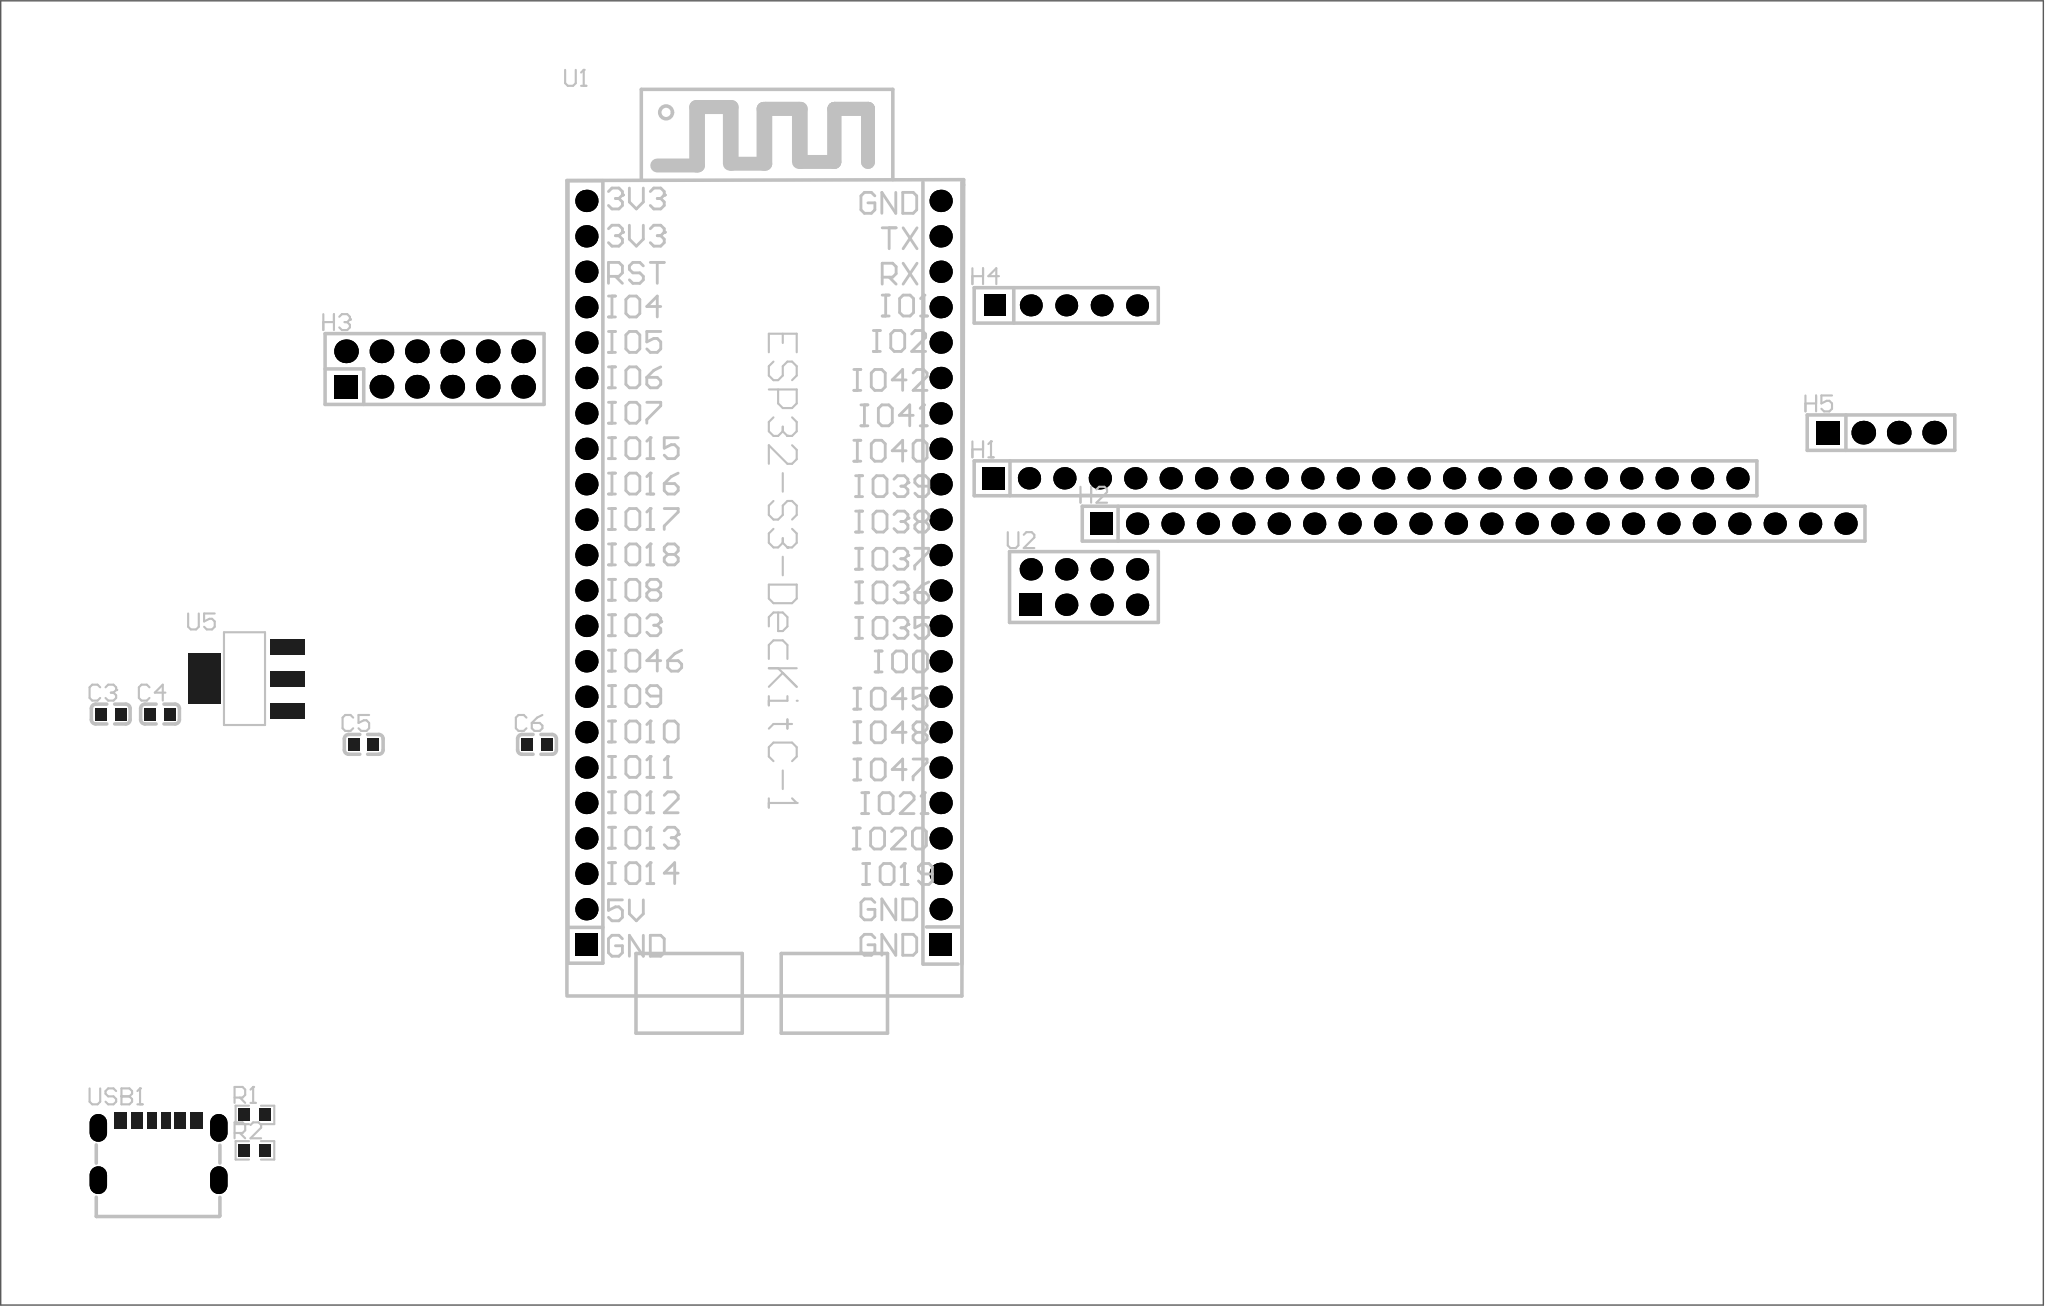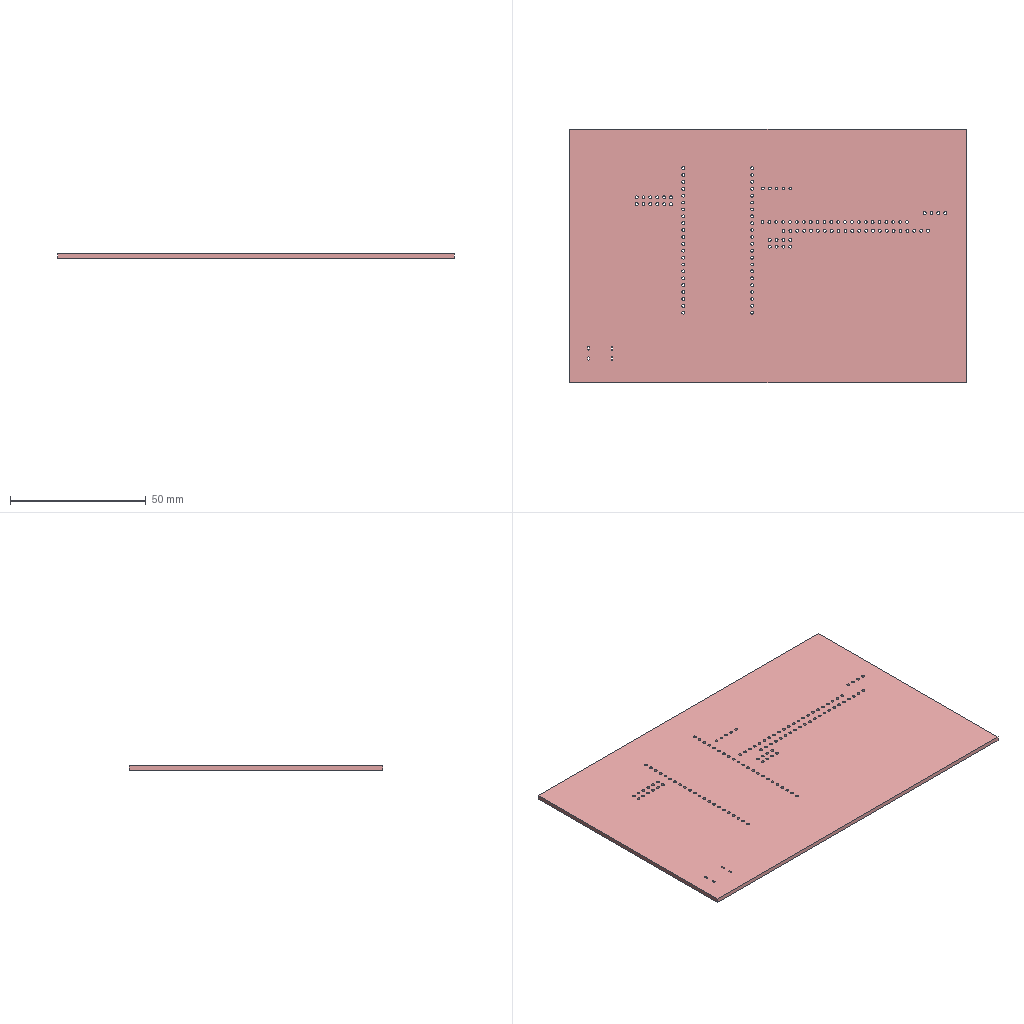Circuit board layout | Altium Designer | box 146.5 x 93.5 x 1.6 mm
Layer stack:
# Altium Designer layer stack of  (unit mm; dielectric type: 0 none, 1 core, 2 prepreg, 3 surface material)
index,name,kind,layer,copper_thickness_mm,dielectric_type,dielectric_thickness_mm,dielectric_material,dielectric_constant
0,Top Paste Mask Layer,other,,,,,,
1,Top Silkscreen Layer,other,,,,,,
2,Top Solder Mask Layer,dielectric,,,3,0.01,,3.3
3,Top Layer,copper,Top Layer,0.035,,,,
4,Dielectric1,dielectric,,,3,1.51,FR4,4.5
5,Bottom Layer,copper,Bottom Layer,0.035,,,,
6,Bottom Solder Mask Layer,dielectric,,,3,0.01,,3.3
7,Bottom Silkscreen Layer,other,,,,,,
8,Bottom Paste Mask Layer,other,,,,,,
# drill layer pairs: low layer,high layer
drill_pair,Top Layer,Bottom Layer
Part placement:
Designator,Comment,Layer,Footprint,Center-X(mm),Center-Y(mm),Rotation
C3,10uF,TopLayer,C0603,77.739,112.237,0
C4,100nF,TopLayer,C0603,81.273,112.237,0
C5,10uF,TopLayer,C0603,95.879,110.063,0
C6,100nF,TopLayer,C0603,108.303,110.063,0
H1,CS-1165SDIG-1*22,TopLayer,HDR-TH_22P-P2.54-V-F,167.709,129.145,0
H2,CS-1165SDIG-1*22,TopLayer,HDR-TH_22P-P2.54-V-F,175.459,125.891,0
H3,LD3320,TopLayer,HDR-TH_12P-P2.54-V-F-R2-C6-S2.54,100.959,136.983,0
H4,SYN6288,TopLayer,HDR-TH_5P-P2.54-V-F,146.249,141.547,0
H5,OLED,TopLayer,HDR-TH_4P-P2.54-V-F,204.669,132.419,0
U1,ESP32-S3-DEVKITC-1-1000MIL,TopLayer,ESP32-S3-DEVKITC-1-1000MIL,124.544,122.37,0
U2,max30102,TopLayer,HDR-TH_8P-P2.54-V-F-R2-C4-S2.54,147.519,121.347,0
U5,AMS1117-3.3,TopLayer,SOT-223-3_L6.5-W3.4-P2.30-LS7.0-BR,87.43,114.778,0
R1,5.1K,TopLayer,R0603,88.079,83.486,0
R2,5.1K,TopLayer,R0603,88.079,80.946,0
USB1,,TopLayer,USB__TYPE-C-6P,81.17,80.946,0
Pad and via stacks:
# Altium Designer via and pad stacks of  (unit mm). Each distinct definition once, with the count of objects using it.
# via: kind,start_layer,end_layer,hole_mm,diameter_mm,mode(0 simple;1 top-mid-bottom;2 full stack),diameter_per_layer,count,example_net
# pad: kind,layer,hole_mm,hole_type(0 round;1 square;2 slot),plating,top_size,top_shape(1 round;2 rect;3 octagon;9 rounded rect),mid_size,bottom_size,mode,footprint,size_per_layer,count,example
pad,Top Layer,0,0,plated,0.8x0.9,2,0.8x0.9,0.8x0.9,0,C0603,,8,C3.2
pad,Top Layer,0,0,plated,2.5x1.1,2,2.5x1.1,2.5x1.1,0,SOT-223-3_L6.5-W3.4-P2.30-LS7.0-BR,,3,U5.1
pad,Top Layer,0,0,plated,2.34x3.6,2,2.34x3.6,2.34x3.6,0,SOT-223-3_L6.5-W3.4-P2.30-LS7.0-BR,,1,U5.4
pad,Top Layer,0,0,plated,0.8065x0.864,2,0.8065x0.864,0.8065x0.864,0,R0603,,4,R1.2
pad,Top Layer,0,0,plated,0.7x1.2,2,0.7x1.2,0.7x1.2,0,USB_ TYPE-C-6P,,2,USB1.A5
pad,Top Layer,0,0,plated,0.8x1.2,2,0.8x1.2,0.8x1.2,0,USB_ TYPE-C-6P,,2,USB1.B9
pad,Top Layer,0,0,plated,0.9x1.2,2,0.9x1.2,0.9x1.2,0,USB_ TYPE-C-6P,,2,USB1.B12
pad,Multi-Layer,1.05,0,plated,1.6x1.6,2,1.6x1.6,1.6x1.6,0,HDR-TH_22P-P2.54-V-F,,2,H1.1
pad,Multi-Layer,1.05,0,plated,1.6x1.6,1,1.6x1.6,1.6x1.6,0,HDR-TH_22P-P2.54-V-F,,42,H1.2
pad,Multi-Layer,1.1,0,plated,1.7x1.7,2,1.7x1.7,1.7x1.7,0,HDR-TH_12P-P2.54-V-F-R2-C6-S2.54,,1,H3.1
pad,Multi-Layer,1.1,0,plated,1.7x1.7,1,1.7x1.7,1.7x1.7,0,HDR-TH_12P-P2.54-V-F-R2-C6-S2.54,,11,H3.2
pad,Multi-Layer,1.02,0,plated,1.575x1.575,1,1.575x1.575,1.575x1.575,0,HDR-TH_5P-P2.54-V-F,,4,H4.5
pad,Multi-Layer,1.02,0,plated,1.575x1.575,2,1.575x1.575,1.575x1.575,0,HDR-TH_5P-P2.54-V-F,,1,H4.1
pad,Multi-Layer,1.1,0,plated,1.7x1.7,2,1.7x1.7,1.7x1.7,0,HDR-TH_4P-P2.54-V-F,,1,H5.1
pad,Multi-Layer,1.1,0,plated,1.7x1.7,1,1.7x1.7,1.7x1.7,0,HDR-TH_4P-P2.54-V-F,,3,H5.2
pad,Multi-Layer,1.05,0,plated,1.6x1.6,1,1.6x1.6,1.6x1.6,0,ESP32-S3-DEVKITC-1-1000MIL,,42,U1.23
pad,Multi-Layer,1.05,0,plated,1.6x1.6,2,1.6x1.6,1.6x1.6,0,ESP32-S3-DEVKITC-1-1000MIL,,2,U1.44
pad,Multi-Layer,1.1,0,plated,1.6x1.6,2,1.6x1.6,1.6x1.6,0,HDR-TH_8P-P2.54-V-F-R2-C4-S2.54,,1,U2.1
pad,Multi-Layer,1.1,0,plated,1.6x1.6,1,1.6x1.6,1.6x1.6,0,HDR-TH_8P-P2.54-V-F-R2-C4-S2.54,,7,U2.2
pad,Multi-Layer,0.6,2,plated,1.25x2,1,1.25x2,1.25x2,0,USB_ TYPE-C-6P,,4,USB1.8